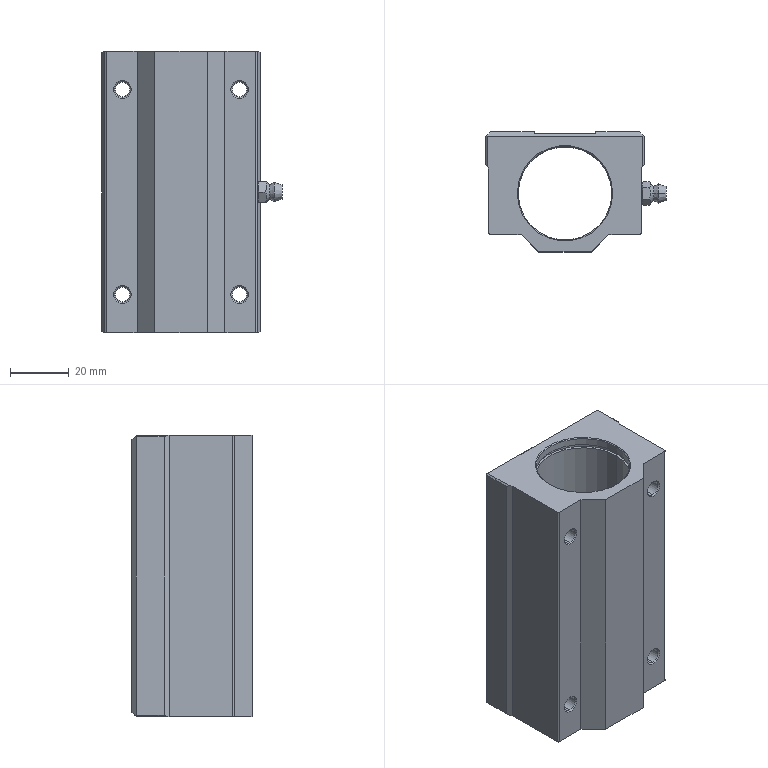Part | SolidWorks | features BaseBody 1 | 1 solid | 97 faces | box 61.5 x 41 x 96 mm | volume 109447 mm3 | plane 41 | cylinder 28 | cone 28 | commonest cylinder face diameters 4.917 x8 5.2 x8 32 x6 33.7 x4 1 x2